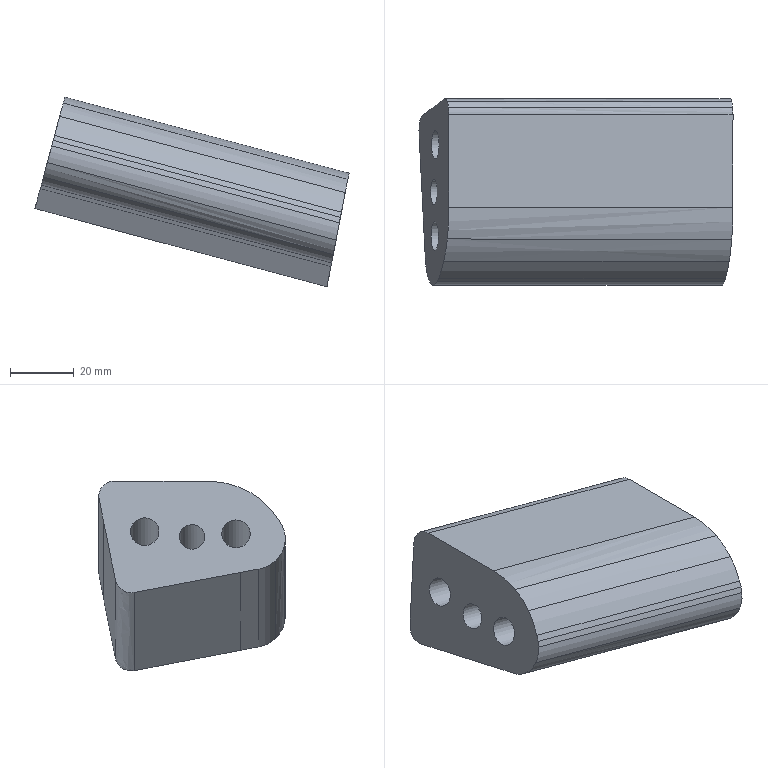Part | NX | features solid 2 | 1 solid | 30 faces | box 98.643 x 58.579 x 59.607 mm | volume 135226 mm3 | spline 16 | plane 8 | cylinder 6 | commonest cylinder face diameters 9.007 x2 14.508 x2 5.1 x1 8 x1
STEP:
#1=CARTESIAN_POINT('',(556.756,-84.584,-6.76));
#2=VERTEX_POINT('',#1);
#3=CARTESIAN_POINT('',(557.921,-84.584,-2.41));
#4=DIRECTION('',(-0.9659,-0.000000134,0.2588));
#5=DIRECTION('',(-0.2588,0.,-0.9659));
#6=AXIS2_PLACEMENT_3D('',#3,#4,#5);
#7=CIRCLE('',#6,4.503);
#8=EDGE_CURVE('',#2,#2,#7,.F.);
#9=ORIENTED_EDGE('',*,*,#8,.F.);
#10=EDGE_LOOP('',(#9));
#11=FACE_BOUND('',#10,.T.);
#12=CARTESIAN_POINT('',(558.279,-91.705,-1.074));
#13=VERTEX_POINT('',#12);
#14=CARTESIAN_POINT('',(557.921,-84.584,-2.41));
#15=DIRECTION('',(-0.9659,-0.000000134,0.2588));
#16=DIRECTION('',(0.04935,-0.9817,0.1842));
#17=AXIS2_PLACEMENT_3D('',#14,#15,#16);
#18=CIRCLE('',#17,7.254);
#19=EDGE_CURVE('',#13,#13,#18,.F.);
#20=ORIENTED_EDGE('',*,*,#19,.T.);
#21=EDGE_LOOP('',(#20));
#22=FACE_BOUND('',#21,.T.);
#23=CARTESIAN_POINT('',(557.921,-84.584,-2.41));
#24=DIRECTION('',(0.9659,0.000000134,-0.2588));
#25=DIRECTION('',(-0.2588,0.,-0.9659));
#26=AXIS2_PLACEMENT_3D('',#23,#24,#25);
#27=PLANE('',#26);
#28=ADVANCED_FACE('',(#11,#22),#27,.T.);
#29=CARTESIAN_POINT('',(583.419,-84.556,-16.752));
#30=VERTEX_POINT('',#29);
#31=CARTESIAN_POINT('',(584.806,-84.584,-9.614));
#32=DIRECTION('',(-0.9816,0.0002628,0.1908));
#33=DIRECTION('',(-0.1908,0.003761,-0.9816));
#34=AXIS2_PLACEMENT_3D('',#31,#32,#33);
#35=ELLIPSE('',#34,7.272,7.254);
#36=EDGE_CURVE('',#30,#30,#35,.F.);
#37=ORIENTED_EDGE('',*,*,#36,.T.);
#38=EDGE_LOOP('',(#37));
#39=FACE_BOUND('',#38,.T.);
#40=ORIENTED_EDGE('',*,*,#19,.F.);
#41=EDGE_LOOP('',(#40));
#42=FACE_BOUND('',#41,.T.);
#43=CARTESIAN_POINT('',(557.921,-84.584,-2.41));
#44=DIRECTION('',(0.9659,0.000000134,-0.2588));
#45=DIRECTION('',(-0.2588,0.,-0.9659));
#46=AXIS2_PLACEMENT_3D('',#43,#44,#45);
#47=CYLINDRICAL_SURFACE('',#46,7.254);
#48=ADVANCED_FACE('',(#39,#42),#47,.F.);
#49=ORIENTED_EDGE('',*,*,#36,.F.);
#50=EDGE_LOOP('',(#49));
#51=FACE_BOUND('',#50,.T.);
#52=CARTESIAN_POINT('',(583.557,-55.874,-16.077));
#53=VERTEX_POINT('',#52);
#54=CARTESIAN_POINT('',(584.945,-55.901,-8.939));
#55=DIRECTION('',(-0.9816,0.0002628,0.1908));
#56=DIRECTION('',(-0.1908,0.003761,-0.9816));
#57=AXIS2_PLACEMENT_3D('',#54,#55,#56);
#58=ELLIPSE('',#57,7.272,7.254);
#59=EDGE_CURVE('',#53,#53,#58,.F.);
#60=ORIENTED_EDGE('',*,*,#59,.F.);
#61=EDGE_LOOP('',(#60));
#62=FACE_BOUND('',#61,.T.);
#63=CARTESIAN_POINT('',(587.981,-44.117,6.663));
#64=VERTEX_POINT('',#63);
#65=CARTESIAN_POINT('',(588.09,-46.498,7.229));
#66=VERTEX_POINT('',#65);
#67=CARTESIAN_POINT('',(587.981,-44.117,6.663));
#68=CARTESIAN_POINT('',(588.053,-44.854,7.038));
#69=CARTESIAN_POINT('',(588.091,-45.668,7.229));
#70=CARTESIAN_POINT('',(588.09,-46.498,7.229));
#71=B_SPLINE_CURVE_WITH_KNOTS('',3,(#67,#68,#69,#70),.UNSPECIFIED.,.F.,.F.,(4,4),(0.,0.002457),.UNSPECIFIED.);
#72=EDGE_CURVE('',#64,#66,#71,.T.);
#73=ORIENTED_EDGE('',*,*,#72,.T.);
#74=CARTESIAN_POINT('',(588.08,-75.541,7.214));
#75=VERTEX_POINT('',#74);
#76=CARTESIAN_POINT('',(588.08,-75.571,7.214));
#77=DIRECTION('',(0.0003677,1.,0.000514));
#78=VECTOR('',#77,1000.);
#79=LINE('',#76,#78);
#80=EDGE_CURVE('',#75,#66,#79,.T.);
#81=ORIENTED_EDGE('',*,*,#80,.F.);
#82=CARTESIAN_POINT('',(587.706,-85.562,5.309));
#83=VERTEX_POINT('',#82);
#84=CARTESIAN_POINT('',(588.08,-75.541,7.214));
#85=CARTESIAN_POINT('',(588.078,-79.006,7.212));
#86=CARTESIAN_POINT('',(587.955,-82.348,6.581));
#87=CARTESIAN_POINT('',(587.706,-85.562,5.309));
#88=B_SPLINE_CURVE_WITH_KNOTS('',3,(#84,#85,#86,#87),.UNSPECIFIED.,.F.,.F.,(4,4),(0.,0.01021),.UNSPECIFIED.);
#89=EDGE_CURVE('',#75,#83,#88,.T.);
#90=ORIENTED_EDGE('',*,*,#89,.T.);
#91=CARTESIAN_POINT('',(586.892,-92.585,1.127));
#92=VERTEX_POINT('',#91);
#93=CARTESIAN_POINT('',(587.706,-85.562,5.309));
#94=CARTESIAN_POINT('',(587.508,-88.136,4.29));
#95=CARTESIAN_POINT('',(587.237,-90.477,2.898));
#96=CARTESIAN_POINT('',(586.892,-92.585,1.127));
#97=B_SPLINE_CURVE_WITH_KNOTS('',3,(#93,#94,#95,#96),.UNSPECIFIED.,.F.,.F.,(4,4),(0.,0.008214),.UNSPECIFIED.);
#98=EDGE_CURVE('',#83,#92,#97,.T.);
#99=ORIENTED_EDGE('',*,*,#98,.T.);
#100=CARTESIAN_POINT('',(585.695,-97.948,-5.022));
#101=VERTEX_POINT('',#100);
#102=CARTESIAN_POINT('',(586.892,-92.585,1.127));
#103=CARTESIAN_POINT('',(586.546,-94.699,-0.6484));
#104=CARTESIAN_POINT('',(586.147,-96.484,-2.701));
#105=CARTESIAN_POINT('',(585.695,-97.948,-5.022));
#106=B_SPLINE_CURVE_WITH_KNOTS('',3,(#102,#103,#104,#105),.UNSPECIFIED.,.F.,.F.,(4,4),(0.,0.008246),.UNSPECIFIED.);
#107=EDGE_CURVE('',#92,#101,#106,.T.);
#108=ORIENTED_EDGE('',*,*,#107,.T.);
#109=CARTESIAN_POINT('',(585.383,-98.902,-6.628));
#110=VERTEX_POINT('',#109);
#111=CARTESIAN_POINT('',(585.695,-97.948,-5.022));
#112=CARTESIAN_POINT('',(585.593,-98.28,-5.549));
#113=CARTESIAN_POINT('',(585.488,-98.598,-6.085));
#114=CARTESIAN_POINT('',(585.383,-98.902,-6.628));
#115=B_SPLINE_CURVE_WITH_KNOTS('',3,(#111,#112,#113,#114),.UNSPECIFIED.,.F.,.F.,(4,4),(0.,0.001895),.UNSPECIFIED.);
#116=EDGE_CURVE('',#101,#110,#115,.T.);
#117=ORIENTED_EDGE('',*,*,#116,.T.);
#118=CARTESIAN_POINT('',(585.05,-99.633,-8.337));
#119=VERTEX_POINT('',#118);
#120=CARTESIAN_POINT('',(585.383,-98.902,-6.628));
#121=CARTESIAN_POINT('',(585.277,-99.207,-7.173));
#122=CARTESIAN_POINT('',(585.166,-99.451,-7.742));
#123=CARTESIAN_POINT('',(585.05,-99.633,-8.337));
#124=B_SPLINE_CURVE_WITH_KNOTS('',3,(#120,#121,#122,#123),.UNSPECIFIED.,.F.,.F.,(4,4),(0.,0.001887),.UNSPECIFIED.);
#125=EDGE_CURVE('',#110,#119,#124,.T.);
#126=ORIENTED_EDGE('',*,*,#125,.T.);
#127=CARTESIAN_POINT('',(584.005,-99.734,-13.713));
#128=VERTEX_POINT('',#127);
#129=CARTESIAN_POINT('',(584.005,-99.734,-13.713));
#130=CARTESIAN_POINT('',(584.349,-100.208,-11.945));
#131=CARTESIAN_POINT('',(584.71,-100.172,-10.087));
#132=CARTESIAN_POINT('',(585.05,-99.633,-8.337));
#133=B_SPLINE_CURVE_WITH_KNOTS('',3,(#129,#130,#131,#132),.UNSPECIFIED.,.F.,.F.,(4,4),(0.,0.00551),.UNSPECIFIED.);
#134=EDGE_CURVE('',#128,#119,#133,.T.);
#135=ORIENTED_EDGE('',*,*,#134,.F.);
#136=CARTESIAN_POINT('',(583.108,-96.945,-18.332));
#137=VERTEX_POINT('',#136);
#138=CARTESIAN_POINT('',(584.005,-99.734,-13.713));
#139=CARTESIAN_POINT('',(583.662,-99.26,-15.479));
#140=CARTESIAN_POINT('',(583.352,-98.295,-17.076));
#141=CARTESIAN_POINT('',(583.108,-96.945,-18.332));
#142=B_SPLINE_CURVE_WITH_KNOTS('',3,(#138,#139,#140,#141),.UNSPECIFIED.,.F.,.F.,(4,4),(0.,0.005502),.UNSPECIFIED.);
#143=EDGE_CURVE('',#128,#137,#142,.T.);
#144=ORIENTED_EDGE('',*,*,#143,.T.);
#145=CARTESIAN_POINT('',(582.61,-91.803,-20.901));
#146=VERTEX_POINT('',#145);
#147=CARTESIAN_POINT('',(583.108,-96.945,-18.332));
#148=CARTESIAN_POINT('',(582.851,-95.518,-19.658));
#149=CARTESIAN_POINT('',(582.678,-93.734,-20.549));
#150=CARTESIAN_POINT('',(582.61,-91.803,-20.901));
#151=B_SPLINE_CURVE_WITH_KNOTS('',3,(#147,#148,#149,#150),.UNSPECIFIED.,.F.,.F.,(4,4),(0.,0.005811),.UNSPECIFIED.);
#152=EDGE_CURVE('',#137,#146,#151,.T.);
#153=ORIENTED_EDGE('',*,*,#152,.T.);
#154=CARTESIAN_POINT('',(582.397,-85.892,-22.005));
#155=VERTEX_POINT('',#154);
#156=CARTESIAN_POINT('',(582.61,-91.803,-20.901));
#157=CARTESIAN_POINT('',(582.541,-89.831,-21.261));
#158=CARTESIAN_POINT('',(582.47,-87.86,-21.628));
#159=CARTESIAN_POINT('',(582.397,-85.892,-22.005));
#160=B_SPLINE_CURVE_WITH_KNOTS('',3,(#156,#157,#158,#159),.UNSPECIFIED.,.F.,.F.,(4,4),(0.,0.006017),.UNSPECIFIED.);
#161=EDGE_CURVE('',#146,#155,#160,.T.);
#162=ORIENTED_EDGE('',*,*,#161,.T.);
#163=CARTESIAN_POINT('',(581.168,-52.586,-28.373));
#164=VERTEX_POINT('',#163);
#165=CARTESIAN_POINT('',(573.42,157.396,-68.523));
#166=DIRECTION('',(-0.03622,0.9816,-0.1877));
#167=VECTOR('',#166,1000.);
#168=LINE('',#165,#167);
#169=EDGE_CURVE('',#155,#164,#168,.T.);
#170=ORIENTED_EDGE('',*,*,#169,.T.);
#171=CARTESIAN_POINT('',(581.924,-46.723,-24.494));
#172=VERTEX_POINT('',#171);
#173=CARTESIAN_POINT('',(581.168,-52.586,-28.373));
#174=CARTESIAN_POINT('',(581.12,-51.29,-28.621));
#175=CARTESIAN_POINT('',(581.23,-48.542,-28.06));
#176=CARTESIAN_POINT('',(581.677,-46.975,-25.766));
#177=CARTESIAN_POINT('',(581.924,-46.723,-24.494));
#178=B_SPLINE_CURVE_WITH_KNOTS('',3,(#173,#174,#175,#176,#177),.UNSPECIFIED.,.F.,.F.,(4,1,4),(0.,0.003905,0.007811),.UNSPECIFIED.);
#179=EDGE_CURVE('',#164,#172,#178,.T.);
#180=ORIENTED_EDGE('',*,*,#179,.T.);
#181=CARTESIAN_POINT('',(584.195,-44.406,-12.814));
#182=VERTEX_POINT('',#181);
#183=CARTESIAN_POINT('',(585.983,-42.581,-3.616));
#184=DIRECTION('',(-0.1873,-0.1911,-0.9635));
#185=VECTOR('',#184,1000.);
#186=LINE('',#183,#185);
#187=EDGE_CURVE('',#182,#172,#186,.T.);
#188=ORIENTED_EDGE('',*,*,#187,.F.);
#189=CARTESIAN_POINT('',(585.604,-42.975,-5.566));
#190=VERTEX_POINT('',#189);
#191=CARTESIAN_POINT('',(584.195,-44.406,-12.814));
#192=CARTESIAN_POINT('',(584.665,-43.926,-10.398));
#193=CARTESIAN_POINT('',(585.134,-43.45,-7.982));
#194=CARTESIAN_POINT('',(585.604,-42.975,-5.566));
#195=B_SPLINE_CURVE_WITH_KNOTS('',3,(#191,#192,#193,#194),.UNSPECIFIED.,.F.,.F.,(4,4),(0.,0.007522),.UNSPECIFIED.);
#196=EDGE_CURVE('',#182,#190,#195,.T.);
#197=ORIENTED_EDGE('',*,*,#196,.T.);
#198=CARTESIAN_POINT('',(587.,-41.572,1.616));
#199=VERTEX_POINT('',#198);
#200=CARTESIAN_POINT('',(585.604,-42.975,-5.566));
#201=CARTESIAN_POINT('',(586.07,-42.505,-3.172));
#202=CARTESIAN_POINT('',(586.535,-42.037,-0.7783));
#203=CARTESIAN_POINT('',(587.,-41.572,1.616));
#204=B_SPLINE_CURVE_WITH_KNOTS('',3,(#200,#201,#202,#203),.UNSPECIFIED.,.F.,.F.,(4,4),(0.,0.007449),.UNSPECIFIED.);
#205=EDGE_CURVE('',#190,#199,#204,.T.);
#206=ORIENTED_EDGE('',*,*,#205,.T.);
#207=CARTESIAN_POINT('',(587.353,-41.584,3.431));
#208=VERTEX_POINT('',#207);
#209=CARTESIAN_POINT('',(587.,-41.572,1.616));
#210=CARTESIAN_POINT('',(587.118,-41.454,2.222));
#211=CARTESIAN_POINT('',(587.236,-41.457,2.827));
#212=CARTESIAN_POINT('',(587.353,-41.584,3.431));
#213=B_SPLINE_CURVE_WITH_KNOTS('',3,(#209,#210,#211,#212),.UNSPECIFIED.,.F.,.F.,(4,4),(0.,0.001849),.UNSPECIFIED.);
#214=EDGE_CURVE('',#199,#208,#213,.T.);
#215=ORIENTED_EDGE('',*,*,#214,.T.);
#216=CARTESIAN_POINT('',(587.677,-42.305,5.095));
#217=VERTEX_POINT('',#216);
#218=CARTESIAN_POINT('',(587.353,-41.584,3.431));
#219=CARTESIAN_POINT('',(587.47,-41.711,4.033));
#220=CARTESIAN_POINT('',(587.578,-41.952,4.588));
#221=CARTESIAN_POINT('',(587.677,-42.305,5.095));
#222=B_SPLINE_CURVE_WITH_KNOTS('',3,(#218,#219,#220,#221),.UNSPECIFIED.,.F.,.F.,(4,4),(0.,0.001842),.UNSPECIFIED.);
#223=EDGE_CURVE('',#208,#217,#222,.T.);
#224=ORIENTED_EDGE('',*,*,#223,.T.);
#225=CARTESIAN_POINT('',(587.677,-42.305,5.095));
#226=CARTESIAN_POINT('',(587.806,-42.767,5.759));
#227=CARTESIAN_POINT('',(587.909,-43.389,6.293));
#228=CARTESIAN_POINT('',(587.981,-44.117,6.663));
#229=B_SPLINE_CURVE_WITH_KNOTS('',3,(#225,#226,#227,#228),.UNSPECIFIED.,.F.,.F.,(4,4),(0.,0.002422),.UNSPECIFIED.);
#230=EDGE_CURVE('',#217,#64,#229,.T.);
#231=ORIENTED_EDGE('',*,*,#230,.T.);
#232=EDGE_LOOP('',(#73,#81,#90,#99,#108,#117,#126,#135,#144,#153,#162,#170,#180,#188,#197,#206,#215,#224,#231));
#233=FACE_BOUND('',#232,.T.);
#234=CARTESIAN_POINT('',(585.102,-70.813,-8.111));
#235=VERTEX_POINT('',#234);
#236=CARTESIAN_POINT('',(584.614,-70.804,-10.62));
#237=DIRECTION('',(-0.9816,0.0002628,0.1908));
#238=DIRECTION('',(0.1908,-0.003761,0.9816));
#239=AXIS2_PLACEMENT_3D('',#236,#237,#238);
#240=ELLIPSE('',#239,2.556,2.55);
#241=EDGE_CURVE('',#235,#235,#240,.F.);
#242=ORIENTED_EDGE('',*,*,#241,.F.);
#243=EDGE_LOOP('',(#242));
#244=FACE_BOUND('',#243,.T.);
#245=CARTESIAN_POINT('',(574.049,158.037,-65.289));
#246=DIRECTION('',(-0.9816,0.0002628,0.1908));
#247=DIRECTION('',(0.1908,0.001526,0.9816));
#248=AXIS2_PLACEMENT_3D('',#245,#246,#247);
#249=PLANE('',#248);
#250=ADVANCED_FACE('',(#51,#62,#233,#244),#249,.F.);
#251=CARTESIAN_POINT('',(493.104,-70.804,9.759));
#252=VERTEX_POINT('',#251);
#253=CARTESIAN_POINT('',(494.139,-70.804,13.623));
#254=DIRECTION('',(-0.9659,-0.000000134,0.2588));
#255=DIRECTION('',(-0.2588,0.,-0.9659));
#256=AXIS2_PLACEMENT_3D('',#253,#254,#255);
#257=CIRCLE('',#256,4.);
#258=EDGE_CURVE('',#252,#252,#257,.T.);
#259=ORIENTED_EDGE('',*,*,#258,.F.);
#260=EDGE_LOOP('',(#259));
#261=FACE_BOUND('',#260,.T.);
#262=CARTESIAN_POINT('',(495.747,-55.901,19.624));
#263=VERTEX_POINT('',#262);
#264=CARTESIAN_POINT('',(494.581,-55.901,15.274));
#265=DIRECTION('',(0.9659,0.000000134,-0.2588));
#266=DIRECTION('',(0.2588,0.,0.9659));
#267=AXIS2_PLACEMENT_3D('',#264,#265,#266);
#268=CIRCLE('',#267,4.503);
#269=EDGE_CURVE('',#263,#263,#268,.T.);
#270=ORIENTED_EDGE('',*,*,#269,.T.);
#271=EDGE_LOOP('',(#270));
#272=FACE_BOUND('',#271,.T.);
#273=CARTESIAN_POINT('',(493.562,-44.406,11.471));
#274=VERTEX_POINT('',#273);
#275=CARTESIAN_POINT('',(495.469,-42.975,18.586));
#276=VERTEX_POINT('',#275);
#277=CARTESIAN_POINT('',(493.562,-44.406,11.471));
#278=CARTESIAN_POINT('',(494.198,-43.926,13.842));
#279=CARTESIAN_POINT('',(494.833,-43.45,16.214));
#280=CARTESIAN_POINT('',(495.469,-42.975,18.586));
#281=B_SPLINE_CURVE_WITH_KNOTS('',3,(#277,#278,#279,#280),.UNSPECIFIED.,.F.,.F.,(4,4),(0.,0.007504),.UNSPECIFIED.);
#282=EDGE_CURVE('',#274,#276,#281,.T.);
#283=ORIENTED_EDGE('',*,*,#282,.F.);
#284=CARTESIAN_POINT('',(490.49,-46.723,0.005664));
#285=VERTEX_POINT('',#284);
#286=CARTESIAN_POINT('',(493.562,-44.406,11.471));
#287=DIRECTION('',(-0.254,-0.1916,-0.948));
#288=VECTOR('',#287,1000.);
#289=LINE('',#286,#288);
#290=EDGE_CURVE('',#274,#285,#289,.T.);
#291=ORIENTED_EDGE('',*,*,#290,.T.);
#292=CARTESIAN_POINT('',(489.47,-52.586,-3.803));
#293=VERTEX_POINT('',#292);
#294=CARTESIAN_POINT('',(490.49,-46.723,0.005664));
#295=CARTESIAN_POINT('',(490.155,-46.976,-1.245));
#296=CARTESIAN_POINT('',(489.553,-48.54,-3.493));
#297=CARTESIAN_POINT('',(489.405,-51.291,-4.046));
#298=CARTESIAN_POINT('',(489.47,-52.586,-3.803));
#299=B_SPLINE_CURVE_WITH_KNOTS('',3,(#294,#295,#296,#297,#298),.UNSPECIFIED.,.F.,.F.,(4,1,4),(0.,0.003902,0.007804),.UNSPECIFIED.);
#300=EDGE_CURVE('',#285,#293,#299,.T.);
#301=ORIENTED_EDGE('',*,*,#300,.T.);
#302=CARTESIAN_POINT('',(491.144,-85.892,2.446));
#303=VERTEX_POINT('',#302);
#304=CARTESIAN_POINT('',(489.47,-52.586,-3.803));
#305=DIRECTION('',(0.04935,-0.9817,0.1842));
#306=VECTOR('',#305,1000.);
#307=LINE('',#304,#306);
#308=EDGE_CURVE('',#293,#303,#307,.T.);
#309=ORIENTED_EDGE('',*,*,#308,.T.);
#310=CARTESIAN_POINT('',(491.435,-91.803,3.529));
#311=VERTEX_POINT('',#310);
#312=CARTESIAN_POINT('',(491.144,-85.892,2.446));
#313=CARTESIAN_POINT('',(491.243,-87.86,2.816));
#314=CARTESIAN_POINT('',(491.34,-89.831,3.177));
#315=CARTESIAN_POINT('',(491.435,-91.803,3.529));
#316=B_SPLINE_CURVE_WITH_KNOTS('',3,(#312,#313,#314,#315),.UNSPECIFIED.,.F.,.F.,(4,4),(0.,0.006016),.UNSPECIFIED.);
#317=EDGE_CURVE('',#303,#311,#316,.T.);
#318=ORIENTED_EDGE('',*,*,#317,.T.);
#319=CARTESIAN_POINT('',(492.11,-96.945,6.051));
#320=VERTEX_POINT('',#319);
#321=CARTESIAN_POINT('',(492.11,-96.945,6.051));
#322=CARTESIAN_POINT('',(491.761,-95.517,4.748));
#323=CARTESIAN_POINT('',(491.527,-93.734,3.874));
#324=CARTESIAN_POINT('',(491.435,-91.803,3.529));
#325=B_SPLINE_CURVE_WITH_KNOTS('',3,(#321,#322,#323,#324),.UNSPECIFIED.,.F.,.F.,(4,4),(0.,0.005808),.UNSPECIFIED.);
#326=EDGE_CURVE('',#320,#311,#325,.T.);
#327=ORIENTED_EDGE('',*,*,#326,.F.);
#328=CARTESIAN_POINT('',(493.325,-99.734,10.584));
#329=VERTEX_POINT('',#328);
#330=CARTESIAN_POINT('',(492.11,-96.945,6.051));
#331=CARTESIAN_POINT('',(492.44,-98.295,7.283));
#332=CARTESIAN_POINT('',(492.86,-99.26,8.85));
#333=CARTESIAN_POINT('',(493.325,-99.734,10.584));
#334=B_SPLINE_CURVE_WITH_KNOTS('',3,(#330,#331,#332,#333),.UNSPECIFIED.,.F.,.F.,(4,4),(0.,0.005492),.UNSPECIFIED.);
#335=EDGE_CURVE('',#320,#329,#334,.T.);
#336=ORIENTED_EDGE('',*,*,#335,.T.);
#337=CARTESIAN_POINT('',(494.739,-99.633,15.862));
#338=VERTEX_POINT('',#337);
#339=CARTESIAN_POINT('',(493.325,-99.734,10.584));
#340=CARTESIAN_POINT('',(493.79,-100.208,12.32));
#341=CARTESIAN_POINT('',(494.279,-100.172,14.144));
#342=CARTESIAN_POINT('',(494.739,-99.633,15.862));
#343=B_SPLINE_CURVE_WITH_KNOTS('',3,(#339,#340,#341,#342),.UNSPECIFIED.,.F.,.F.,(4,4),(0.,0.005497),.UNSPECIFIED.);
#344=EDGE_CURVE('',#329,#338,#343,.T.);
#345=ORIENTED_EDGE('',*,*,#344,.T.);
#346=CARTESIAN_POINT('',(495.188,-98.902,17.539));
#347=VERTEX_POINT('',#346);
#348=CARTESIAN_POINT('',(494.739,-99.633,15.862));
#349=CARTESIAN_POINT('',(494.896,-99.451,16.446));
#350=CARTESIAN_POINT('',(495.045,-99.207,17.005));
#351=CARTESIAN_POINT('',(495.188,-98.902,17.539));
#352=B_SPLINE_CURVE_WITH_KNOTS('',3,(#348,#349,#350,#351),.UNSPECIFIED.,.F.,.F.,(4,4),(0.,0.001884),.UNSPECIFIED.);
#353=EDGE_CURVE('',#338,#347,#352,.T.);
#354=ORIENTED_EDGE('',*,*,#353,.T.);
#355=CARTESIAN_POINT('',(495.611,-97.948,19.116));
#356=VERTEX_POINT('',#355);
#357=CARTESIAN_POINT('',(495.188,-98.902,17.539));
#358=CARTESIAN_POINT('',(495.331,-98.598,18.073));
#359=CARTESIAN_POINT('',(495.472,-98.28,18.598));
#360=CARTESIAN_POINT('',(495.611,-97.948,19.116));
#361=B_SPLINE_CURVE_WITH_KNOTS('',3,(#357,#358,#359,#360),.UNSPECIFIED.,.F.,.F.,(4,4),(0.,0.001891),.UNSPECIFIED.);
#362=EDGE_CURVE('',#347,#356,#361,.T.);
#363=ORIENTED_EDGE('',*,*,#362,.T.);
#364=CARTESIAN_POINT('',(497.228,-92.585,25.152));
#365=VERTEX_POINT('',#364);
#366=CARTESIAN_POINT('',(495.611,-97.948,19.116));
#367=CARTESIAN_POINT('',(496.222,-96.483,21.396));
#368=CARTESIAN_POINT('',(496.762,-94.698,23.41));
#369=CARTESIAN_POINT('',(497.228,-92.585,25.152));
#370=B_SPLINE_CURVE_WITH_KNOTS('',3,(#366,#367,#368,#369),.UNSPECIFIED.,.F.,.F.,(4,4),(0.,0.008235),.UNSPECIFIED.);
#371=EDGE_CURVE('',#356,#365,#370,.T.);
#372=ORIENTED_EDGE('',*,*,#371,.T.);
#373=CARTESIAN_POINT('',(498.328,-85.563,29.257));
#374=VERTEX_POINT('',#373);
#375=CARTESIAN_POINT('',(497.228,-92.585,25.152));
#376=CARTESIAN_POINT('',(497.694,-90.477,26.891));
#377=CARTESIAN_POINT('',(498.061,-88.135,28.258));
#378=CARTESIAN_POINT('',(498.328,-85.563,29.257));
#379=B_SPLINE_CURVE_WITH_KNOTS('',3,(#375,#376,#377,#378),.UNSPECIFIED.,.F.,.F.,(4,4),(0.,0.008209),.UNSPECIFIED.);
#380=EDGE_CURVE('',#365,#374,#379,.T.);
#381=ORIENTED_EDGE('',*,*,#380,.T.);
#382=CARTESIAN_POINT('',(498.83,-75.541,31.128));
#383=VERTEX_POINT('',#382);
#384=CARTESIAN_POINT('',(498.83,-75.541,31.128));
#385=CARTESIAN_POINT('',(498.829,-79.006,31.127));
#386=CARTESIAN_POINT('',(498.663,-82.347,30.507));
#387=CARTESIAN_POINT('',(498.328,-85.563,29.257));
#388=B_SPLINE_CURVE_WITH_KNOTS('',3,(#384,#385,#386,#387),.UNSPECIFIED.,.F.,.F.,(4,4),(0.,0.01021),.UNSPECIFIED.);
#389=EDGE_CURVE('',#383,#374,#388,.T.);
#390=ORIENTED_EDGE('',*,*,#389,.F.);
#391=CARTESIAN_POINT('',(498.834,-46.498,31.145));
#392=VERTEX_POINT('',#391);
#393=CARTESIAN_POINT('',(498.83,-75.541,31.128));
#394=DIRECTION('',(0.000153,1.,0.0005715));
#395=VECTOR('',#394,1000.);
#396=LINE('',#393,#395);
#397=EDGE_CURVE('',#383,#392,#396,.T.);
#398=ORIENTED_EDGE('',*,*,#397,.T.);
#399=CARTESIAN_POINT('',(498.685,-44.117,30.589));
#400=VERTEX_POINT('',#399);
#401=CARTESIAN_POINT('',(498.834,-46.498,31.145));
#402=CARTESIAN_POINT('',(498.834,-45.668,31.146));
#403=CARTESIAN_POINT('',(498.784,-44.855,30.957));
#404=CARTESIAN_POINT('',(498.685,-44.117,30.589));
#405=B_SPLINE_CURVE_WITH_KNOTS('',3,(#401,#402,#403,#404),.UNSPECIFIED.,.F.,.F.,(4,4),(0.,0.002456),.UNSPECIFIED.);
#406=EDGE_CURVE('',#392,#400,#405,.T.);
#407=ORIENTED_EDGE('',*,*,#406,.T.);
#408=CARTESIAN_POINT('',(498.273,-42.305,29.051));
#409=VERTEX_POINT('',#408);
#410=CARTESIAN_POINT('',(498.685,-44.117,30.589));
#411=CARTESIAN_POINT('',(498.588,-43.39,30.227));
#412=CARTESIAN_POINT('',(498.448,-42.767,29.703));
#413=CARTESIAN_POINT('',(498.273,-42.305,29.051));
#414=B_SPLINE_CURVE_WITH_KNOTS('',3,(#410,#411,#412,#413),.UNSPECIFIED.,.F.,.F.,(4,4),(0.,0.00242),.UNSPECIFIED.);
#415=EDGE_CURVE('',#400,#409,#414,.T.);
#416=ORIENTED_EDGE('',*,*,#415,.T.);
#417=CARTESIAN_POINT('',(497.835,-41.584,27.417));
#418=VERTEX_POINT('',#417);
#419=CARTESIAN_POINT('',(498.273,-42.305,29.051));
#420=CARTESIAN_POINT('',(498.14,-41.952,28.553));
#421=CARTESIAN_POINT('',(497.994,-41.711,28.008));
#422=CARTESIAN_POINT('',(497.835,-41.584,27.417));
#423=B_SPLINE_CURVE_WITH_KNOTS('',3,(#419,#420,#421,#422),.UNSPECIFIED.,.F.,.F.,(4,4),(0.,0.001839),.UNSPECIFIED.);
#424=EDGE_CURVE('',#409,#418,#423,.T.);
#425=ORIENTED_EDGE('',*,*,#424,.T.);
#426=CARTESIAN_POINT('',(497.358,-41.572,25.636));
#427=VERTEX_POINT('',#426);
#428=CARTESIAN_POINT('',(497.835,-41.584,27.417));
#429=CARTESIAN_POINT('',(497.676,-41.457,26.824));
#430=CARTESIAN_POINT('',(497.517,-41.454,26.23));
#431=CARTESIAN_POINT('',(497.358,-41.572,25.636));
#432=B_SPLINE_CURVE_WITH_KNOTS('',3,(#428,#429,#430,#431),.UNSPECIFIED.,.F.,.F.,(4,4),(0.,0.001844),.UNSPECIFIED.);
#433=EDGE_CURVE('',#418,#427,#432,.T.);
#434=ORIENTED_EDGE('',*,*,#433,.T.);
#435=CARTESIAN_POINT('',(497.358,-41.572,25.636));
#436=CARTESIAN_POINT('',(496.728,-42.037,23.285));
#437=CARTESIAN_POINT('',(496.099,-42.505,20.935));
#438=CARTESIAN_POINT('',(495.469,-42.975,18.586));
#439=B_SPLINE_CURVE_WITH_KNOTS('',3,(#435,#436,#437,#438),.UNSPECIFIED.,.F.,.F.,(4,4),(0.,0.007432),.UNSPECIFIED.);
#440=EDGE_CURVE('',#427,#276,#439,.T.);
#441=ORIENTED_EDGE('',*,*,#440,.T.);
#442=EDGE_LOOP('',(#283,#291,#301,#309,#318,#327,#336,#345,#354,#363,#372,#381,#390,#398,#407,#416,#425,#434,#441));
#443=FACE_BOUND('',#442,.T.);
#444=CARTESIAN_POINT('',(495.569,-84.584,18.96));
#445=VERTEX_POINT('',#444);
#446=CARTESIAN_POINT('',(494.404,-84.584,14.61));
#447=DIRECTION('',(0.9659,0.000000134,-0.2588));
#448=DIRECTION('',(0.2588,0.,0.9659));
#449=AXIS2_PLACEMENT_3D('',#446,#447,#448);
#450=CIRCLE('',#449,4.503);
#451=EDGE_CURVE('',#445,#445,#450,.T.);
#452=ORIENTED_EDGE('',*,*,#451,.T.);
#453=EDGE_LOOP('',(#452));
#454=FACE_BOUND('',#453,.T.);
#455=CARTESIAN_POINT('',(327.709,4.191,-607.503));
#456=DIRECTION('',(-0.9659,-0.000000134,0.2588));
#457=DIRECTION('',(0.2588,0.,0.9659));
#458=AXIS2_PLACEMENT_3D('',#455,#456,#457);
#459=PLANE('',#458);
#460=ADVANCED_FACE('',(#261,#272,#443,#454),#459,.T.);
#461=ORIENTED_EDGE('',*,*,#451,.F.);
#462=EDGE_LOOP('',(#461));
#463=FACE_BOUND('',#462,.T.);
#464=ORIENTED_EDGE('',*,*,#8,.T.);
#465=EDGE_LOOP('',(#464));
#466=FACE_BOUND('',#465,.T.);
#467=CARTESIAN_POINT('',(607.183,-84.584,-15.61));
#468=DIRECTION('',(-0.9659,-0.000000134,0.2588));
#469=DIRECTION('',(0.2588,0.,0.9659));
#470=AXIS2_PLACEMENT_3D('',#467,#468,#469);
#471=CYLINDRICAL_SURFACE('',#470,4.503);
#472=ADVANCED_FACE('',(#463,#466),#471,.F.);
#473=CARTESIAN_POINT('',(457.154,-46.498,42.313));
#474=DIRECTION('',(0.9659,0.000000134,-0.2588));
#475=VECTOR('',#474,1000.);
#476=LINE('',#473,#475);
#477=EDGE_CURVE('',#66,#392,#476,.F.);
#478=ORIENTED_EDGE('',*,*,#477,.T.);
#479=ORIENTED_EDGE('',*,*,#397,.F.);
#480=CARTESIAN_POINT('',(457.088,-75.541,42.313));
#481=DIRECTION('',(0.9659,0.000000134,-0.2588));
#482=VECTOR('',#481,1000.);
#483=LINE('',#480,#482);
#484=EDGE_CURVE('',#75,#383,#483,.F.);
#485=ORIENTED_EDGE('',*,*,#484,.F.);
#486=ORIENTED_EDGE('',*,*,#80,.T.);
#487=EDGE_LOOP('',(#478,#479,#485,#486));
#488=FACE_BOUND('',#487,.T.);
#489=CARTESIAN_POINT('',(457.088,-75.541,42.313));
#490=DIRECTION('',(0.2588,-0.0005916,0.9659));
#491=DIRECTION('',(0.9659,0.,-0.2588));
#492=AXIS2_PLACEMENT_3D('',#489,#490,#491);
#493=PLANE('',#492);
#494=ADVANCED_FACE('',(#488),#493,.T.);
#495=CARTESIAN_POINT('',(455.12,-41.584,38.862));
#496=DIRECTION('',(0.9659,0.000000134,-0.2588));
#497=VECTOR('',#496,1000.);
#498=LINE('',#495,#497);
#499=EDGE_CURVE('',#208,#418,#498,.F.);
#500=ORIENTED_EDGE('',*,*,#499,.T.);
#501=ORIENTED_EDGE('',*,*,#424,.F.);
#502=CARTESIAN_POINT('',(455.997,-42.305,40.379));
#503=DIRECTION('',(0.9659,0.000000134,-0.2588));
#504=VECTOR('',#503,1000.);
#505=LINE('',#502,#504);
#506=EDGE_CURVE('',#217,#409,#505,.F.);
#507=ORIENTED_EDGE('',*,*,#506,.F.);
#508=ORIENTED_EDGE('',*,*,#223,.F.);
#509=EDGE_LOOP('',(#500,#501,#507,#508));
#510=FACE_BOUND('',#509,.T.);
#511=CARTESIAN_POINT('',(497.733,-42.305,29.195));
#512=CARTESIAN_POINT('',(588.77,-42.305,4.802));
#513=CARTESIAN_POINT('',(497.46,-41.956,28.741));
#514=CARTESIAN_POINT('',(588.497,-41.956,4.347));
#515=CARTESIAN_POINT('',(497.16,-41.709,28.223));
#516=CARTESIAN_POINT('',(588.197,-41.709,3.829));
#517=CARTESIAN_POINT('',(496.856,-41.584,27.679));
#518=CARTESIAN_POINT('',(587.893,-41.584,3.286));
#519=B_SPLINE_SURFACE_WITH_KNOTS('',3,1,((#511,#512),(#513,#514),(#515,#516),(#517,#518)),.SURF_OF_LINEAR_EXTRUSION.,.F.,.F.,.F.,(4,4),(2,2),(6.091,6.476),(0.,1.),.PIECEWISE_BEZIER_KNOTS.);
#520=ADVANCED_FACE('',(#510),#519,.F.);
#521=ORIENTED_EDGE('',*,*,#506,.T.);
#522=ORIENTED_EDGE('',*,*,#415,.F.);
#523=CARTESIAN_POINT('',(456.849,-44.117,41.799));
#524=DIRECTION('',(0.9659,0.000000134,-0.2588));
#525=VECTOR('',#524,1000.);
#526=LINE('',#523,#525);
#527=EDGE_CURVE('',#64,#400,#526,.F.);
#528=ORIENTED_EDGE('',*,*,#527,.F.);
#529=ORIENTED_EDGE('',*,*,#230,.F.);
#530=EDGE_LOOP('',(#521,#522,#528,#529));
#531=FACE_BOUND('',#530,.T.);
#532=CARTESIAN_POINT('',(498.146,-44.117,30.734));
#533=CARTESIAN_POINT('',(589.068,-44.117,6.371));
#534=CARTESIAN_POINT('',(497.945,-43.388,30.398));
#535=CARTESIAN_POINT('',(588.867,-43.388,6.035));
#536=CARTESIAN_POINT('',(497.65,-42.76,29.905));
#537=CARTESIAN_POINT('',(588.571,-42.76,5.542));
#538=CARTESIAN_POINT('',(497.294,-42.305,29.313));
#539=CARTESIAN_POINT('',(588.216,-42.305,4.951));
#540=B_SPLINE_SURFACE_WITH_KNOTS('',3,1,((#532,#533),(#534,#535),(#536,#537),(#538,#539)),.SURF_OF_LINEAR_EXTRUSION.,.F.,.F.,.F.,(4,4),(2,2),(0.7564,1.252),(0.,1.),.PIECEWISE_BEZIER_KNOTS.);
#541=ADVANCED_FACE('',(#531),#540,.F.);
#542=ORIENTED_EDGE('',*,*,#527,.T.);
#543=ORIENTED_EDGE('',*,*,#406,.F.);
#544=ORIENTED_EDGE('',*,*,#477,.F.);
#545=ORIENTED_EDGE('',*,*,#72,.F.);
#546=EDGE_LOOP('',(#542,#543,#544,#545));
#547=FACE_BOUND('',#546,.T.);
#548=CARTESIAN_POINT('',(498.296,-46.498,31.289));
#549=CARTESIAN_POINT('',(588.822,-46.498,7.033));
#550=CARTESIAN_POINT('',(498.298,-45.671,31.289));
#551=CARTESIAN_POINT('',(588.824,-45.671,7.033));
#552=CARTESIAN_POINT('',(498.192,-44.845,31.111));
#553=CARTESIAN_POINT('',(588.718,-44.845,6.855));
#554=CARTESIAN_POINT('',(497.992,-44.117,30.775));
#555=CARTESIAN_POINT('',(588.517,-44.117,6.519));
#556=B_SPLINE_SURFACE_WITH_KNOTS('',3,1,((#548,#549),(#550,#551),(#552,#553),(#554,#555)),.SURF_OF_LINEAR_EXTRUSION.,.F.,.F.,.F.,(4,4),(2,2),(0.2624,0.7564),(0.,1.),.PIECEWISE_BEZIER_KNOTS.);
#557=ADVANCED_FACE('',(#547),#556,.F.);
#558=ORIENTED_EDGE('',*,*,#484,.T.);
#559=ORIENTED_EDGE('',*,*,#389,.T.);
#560=CARTESIAN_POINT('',(456.027,-85.563,40.592));
#561=DIRECTION('',(0.9659,0.000000134,-0.2588));
#562=VECTOR('',#561,1000.);
#563=LINE('',#560,#562);
#564=EDGE_CURVE('',#83,#374,#563,.F.);
#565=ORIENTED_EDGE('',*,*,#564,.F.);
#566=ORIENTED_EDGE('',*,*,#89,.F.);
#567=EDGE_LOOP('',(#558,#559,#565,#566));
#568=FACE_BOUND('',#567,.T.);
#569=CARTESIAN_POINT('',(497.229,-85.563,29.552));
#570=CARTESIAN_POINT('',(588.246,-85.562,5.164));
#571=CARTESIAN_POINT('',(497.92,-82.399,30.684));
#572=CARTESIAN_POINT('',(588.936,-82.399,6.296));
#573=CARTESIAN_POINT('',(498.282,-78.971,31.273));
#574=CARTESIAN_POINT('',(589.299,-78.971,6.885));
#575=CARTESIAN_POINT('',(498.29,-75.541,31.273));
#576=CARTESIAN_POINT('',(589.307,-75.541,6.885));
#577=B_SPLINE_SURFACE_WITH_KNOTS('',3,1,((#569,#570),(#571,#572),(#573,#574),(#575,#576)),.SURF_OF_LINEAR_EXTRUSION.,.F.,.F.,.F.,(4,4),(2,2),(6.085,6.481),(0.,1.),.PIECEWISE_BEZIER_KNOTS.);
#578=ADVANCED_FACE('',(#568),#577,.F.);
#579=ORIENTED_EDGE('',*,*,#564,.T.);
#580=ORIENTED_EDGE('',*,*,#380,.F.);
#581=CARTESIAN_POINT('',(453.915,-92.585,36.758));
#582=DIRECTION('',(0.9659,0.000000134,-0.2588));
#583=VECTOR('',#582,1000.);
#584=LINE('',#581,#583);
#585=EDGE_CURVE('',#92,#365,#584,.F.);
#586=ORIENTED_EDGE('',*,*,#585,.F.);
#587=ORIENTED_EDGE('',*,*,#98,.F.);
#588=EDGE_LOOP('',(#579,#580,#586,#587));
#589=FACE_BOUND('',#588,.T.);
#590=CARTESIAN_POINT('',(495.673,-92.585,25.569));
#591=CARTESIAN_POINT('',(587.436,-92.585,0.9813));
#592=CARTESIAN_POINT('',(496.511,-90.499,27.188));
#593=CARTESIAN_POINT('',(588.274,-90.499,2.6));
#594=CARTESIAN_POINT('',(497.227,-88.118,28.488));
#595=CARTESIAN_POINT('',(588.99,-88.118,3.901));
#596=CARTESIAN_POINT('',(497.784,-85.563,29.403));
#597=CARTESIAN_POINT('',(589.548,-85.562,4.815));
#598=B_SPLINE_SURFACE_WITH_KNOTS('',3,1,((#590,#591),(#592,#593),(#594,#595),(#596,#597)),.SURF_OF_LINEAR_EXTRUSION.,.F.,.F.,.F.,(4,4),(2,2),(6.122,6.445),(0.,1.),.PIECEWISE_BEZIER_KNOTS.);
#599=ADVANCED_FACE('',(#589),#598,.F.);
#600=ORIENTED_EDGE('',*,*,#585,.T.);
#601=ORIENTED_EDGE('',*,*,#371,.F.);
#602=CARTESIAN_POINT('',(451.463,-97.948,30.945));
#603=DIRECTION('',(0.9659,0.000000134,-0.2588));
#604=VECTOR('',#603,1000.);
#605=LINE('',#602,#604);
#606=EDGE_CURVE('',#101,#356,#605,.F.);
#607=ORIENTED_EDGE('',*,*,#606,.F.);
#608=ORIENTED_EDGE('',*,*,#107,.F.);
#609=EDGE_LOOP('',(#600,#601,#607,#608));
#610=FACE_BOUND('',#609,.T.);
#611=CARTESIAN_POINT('',(494.231,-97.948,19.486));
#612=CARTESIAN_POINT('',(586.241,-97.948,-5.168));
#613=CARTESIAN_POINT('',(495.013,-96.49,21.709));
#614=CARTESIAN_POINT('',(587.023,-96.489,-2.945));
#615=CARTESIAN_POINT('',(495.844,-94.672,23.679));
#616=CARTESIAN_POINT('',(587.854,-94.672,-0.975));
#617=CARTESIAN_POINT('',(496.683,-92.585,25.298));
#618=CARTESIAN_POINT('',(588.693,-92.585,0.6445));
#619=B_SPLINE_SURFACE_WITH_KNOTS('',3,1,((#611,#612),(#613,#614),(#615,#616),(#617,#618)),.SURF_OF_LINEAR_EXTRUSION.,.F.,.F.,.F.,(4,4),(2,2),(6.125,6.441),(0.,1.),.PIECEWISE_BEZIER_KNOTS.);
#620=ADVANCED_FACE('',(#610),#619,.F.);
#621=ORIENTED_EDGE('',*,*,#606,.T.);
#622=ORIENTED_EDGE('',*,*,#362,.F.);
#623=CARTESIAN_POINT('',(450.945,-98.902,29.394));
#624=DIRECTION('',(0.9659,0.000000134,-0.2588));
#625=VECTOR('',#624,1000.);
#626=LINE('',#623,#625);
#627=EDGE_CURVE('',#110,#347,#626,.F.);
#628=ORIENTED_EDGE('',*,*,#627,.F.);
#629=ORIENTED_EDGE('',*,*,#116,.F.);
#630=EDGE_LOOP('',(#621,#622,#628,#629));
#631=FACE_BOUND('',#630,.T.);
#632=CARTESIAN_POINT('',(494.551,-98.902,17.71));
#633=CARTESIAN_POINT('',(585.924,-98.902,-6.774));
#634=CARTESIAN_POINT('',(494.718,-98.598,18.237));
#635=CARTESIAN_POINT('',(586.091,-98.598,-6.246));
#636=CARTESIAN_POINT('',(494.891,-98.28,18.755));
#637=CARTESIAN_POINT('',(586.264,-98.28,-5.729));
#638=CARTESIAN_POINT('',(495.069,-97.948,19.261));
#639=CARTESIAN_POINT('',(586.442,-97.948,-5.222));
#640=B_SPLINE_SURFACE_WITH_KNOTS('',3,1,((#632,#633),(#634,#635),(#636,#637),(#638,#639)),.SURF_OF_LINEAR_EXTRUSION.,.F.,.F.,.F.,(4,4),(2,2),(6.254,6.312),(0.,1.),.PIECEWISE_BEZIER_KNOTS.);
#641=ADVANCED_FACE('',(#631),#640,.F.);
#642=ORIENTED_EDGE('',*,*,#627,.T.);
#643=ORIENTED_EDGE('',*,*,#353,.F.);
#644=CARTESIAN_POINT('',(450.45,-99.634,27.73));
#645=DIRECTION('',(0.9659,0.000000134,-0.2588));
#646=VECTOR('',#645,1000.);
#647=LINE('',#644,#646);
#648=EDGE_CURVE('',#119,#338,#647,.F.);
#649=ORIENTED_EDGE('',*,*,#648,.F.);
#650=ORIENTED_EDGE('',*,*,#125,.F.);
#651=EDGE_LOOP('',(#642,#643,#649,#650));
#652=FACE_BOUND('',#651,.T.);
#653=CARTESIAN_POINT('',(494.151,-99.633,16.02));
#654=CARTESIAN_POINT('',(585.593,-99.633,-8.482));
#655=CARTESIAN_POINT('',(494.314,-99.451,16.6));
#656=CARTESIAN_POINT('',(585.755,-99.451,-7.902));
#657=CARTESIAN_POINT('',(494.48,-99.206,17.159));
#658=CARTESIAN_POINT('',(585.921,-99.206,-7.343));
#659=CARTESIAN_POINT('',(494.646,-98.902,17.684));
#660=CARTESIAN_POINT('',(586.087,-98.902,-6.817));
#661=B_SPLINE_SURFACE_WITH_KNOTS('',3,1,((#653,#654),(#655,#656),(#657,#658),(#659,#660)),.SURF_OF_LINEAR_EXTRUSION.,.F.,.F.,.F.,(4,4),(2,2),(6.178,6.389),(0.,1.),.PIECEWISE_BEZIER_KNOTS.);
#662=ADVANCED_FACE('',(#652),#661,.F.);
#663=ORIENTED_EDGE('',*,*,#648,.T.);
#664=ORIENTED_EDGE('',*,*,#344,.F.);
#665=CARTESIAN_POINT('',(449.213,-99.734,22.404));
#666=DIRECTION('',(0.9659,0.000000134,-0.2588));
#667=VECTOR('',#666,1000.);
#668=LINE('',#665,#667);
#669=EDGE_CURVE('',#128,#329,#668,.F.);
#670=ORIENTED_EDGE('',*,*,#669,.F.);
#671=ORIENTED_EDGE('',*,*,#134,.T.);
#672=EDGE_LOOP('',(#663,#664,#670,#671));
#673=FACE_BOUND('',#672,.T.);
#674=CARTESIAN_POINT('',(492.781,-99.734,10.73));
#675=CARTESIAN_POINT('',(584.553,-99.734,-13.86));
#676=CARTESIAN_POINT('',(493.108,-100.204,12.486));
#677=CARTESIAN_POINT('',(584.881,-100.204,-12.105));
#678=CARTESIAN_POINT('',(493.542,-100.169,14.354));
#679=CARTESIAN_POINT('',(585.314,-100.169,-10.237));
#680=CARTESIAN_POINT('',(494.018,-99.633,16.056));
#681=CARTESIAN_POINT('',(585.79,-99.633,-8.535));
#682=B_SPLINE_SURFACE_WITH_KNOTS('',3,1,((#674,#675),(#676,#677),(#678,#679),(#680,#681)),.SURF_OF_LINEAR_EXTRUSION.,.F.,.F.,.F.,(4,4),(2,2),(6.004,6.562),(0.,1.),.PIECEWISE_BEZIER_KNOTS.);
#683=ADVANCED_FACE('',(#673),#682,.F.);
#684=ORIENTED_EDGE('',*,*,#669,.T.);
#685=ORIENTED_EDGE('',*,*,#335,.F.);
#686=CARTESIAN_POINT('',(448.336,-96.945,17.78));
#687=DIRECTION('',(0.9659,0.000000134,-0.2588));
#688=VECTOR('',#687,1000.);
#689=LINE('',#686,#688);
#690=EDGE_CURVE('',#137,#320,#689,.F.);
#691=ORIENTED_EDGE('',*,*,#690,.F.);
#692=ORIENTED_EDGE('',*,*,#143,.F.);
#693=EDGE_LOOP('',(#684,#685,#691,#692));
#694=FACE_BOUND('',#693,.T.);
#695=CARTESIAN_POINT('',(491.564,-96.945,6.198));
#696=CARTESIAN_POINT('',(583.675,-96.945,-18.483));
#697=CARTESIAN_POINT('',(491.806,-98.286,7.444));
#698=CARTESIAN_POINT('',(583.917,-98.286,-17.237));
#699=CARTESIAN_POINT('',(492.113,-99.264,9.065));
#700=CARTESIAN_POINT('',(584.224,-99.264,-15.616));
#701=CARTESIAN_POINT('',(492.441,-99.734,10.821));
#702=CARTESIAN_POINT('',(584.551,-99.734,-13.86));
#703=B_SPLINE_SURFACE_WITH_KNOTS('',3,1,((#695,#696),(#697,#698),(#699,#700),(#701,#702)),.SURF_OF_LINEAR_EXTRUSION.,.F.,.F.,.F.,(4,4),(2,2),(6.006,6.561),(0.,1.),.PIECEWISE_BEZIER_KNOTS.);
#704=ADVANCED_FACE('',(#694),#703,.F.);
#705=ORIENTED_EDGE('',*,*,#690,.T.);
#706=ORIENTED_EDGE('',*,*,#326,.T.);
#707=CARTESIAN_POINT('',(447.838,-91.803,15.211));
#708=DIRECTION('',(0.9659,0.000000134,-0.2588));
#709=VECTOR('',#708,1000.);
#710=LINE('',#707,#709);
#711=EDGE_CURVE('',#146,#311,#710,.F.);
#712=ORIENTED_EDGE('',*,*,#711,.F.);
#713=ORIENTED_EDGE('',*,*,#152,.F.);
#714=EDGE_LOOP('',(#705,#706,#712,#713));
#715=FACE_BOUND('',#714,.T.);
#716=CARTESIAN_POINT('',(490.888,-91.803,3.676));
#717=CARTESIAN_POINT('',(582.61,-91.803,-20.901));
#718=CARTESIAN_POINT('',(490.955,-93.72,4.025));
#719=CARTESIAN_POINT('',(582.678,-93.72,-20.552));
#720=CARTESIAN_POINT('',(491.13,-95.529,4.929));
#721=CARTESIAN_POINT('',(582.853,-95.529,-19.648));
#722=CARTESIAN_POINT('',(491.386,-96.945,6.245));
#723=CARTESIAN_POINT('',(583.108,-96.945,-18.332));
#724=B_SPLINE_SURFACE_WITH_KNOTS('',3,1,((#716,#717),(#718,#719),(#720,#721),(#722,#723)),.SURF_OF_LINEAR_EXTRUSION.,.F.,.F.,.F.,(4,4),(2,2),(5.996,6.571),(0.,1.),.PIECEWISE_BEZIER_KNOTS.);
#725=ADVANCED_FACE('',(#715),#724,.F.);
#726=ORIENTED_EDGE('',*,*,#711,.T.);
#727=ORIENTED_EDGE('',*,*,#317,.F.);
#728=CARTESIAN_POINT('',(447.625,-85.892,14.107));
#729=DIRECTION('',(0.9659,0.000000134,-0.2588));
#730=VECTOR('',#729,1000.);
#731=LINE('',#728,#730);
#732=EDGE_CURVE('',#155,#303,#731,.F.);
#733=ORIENTED_EDGE('',*,*,#732,.F.);
#734=ORIENTED_EDGE('',*,*,#161,.F.);
#735=EDGE_LOOP('',(#726,#727,#733,#734));
#736=FACE_BOUND('',#735,.T.);
#737=CARTESIAN_POINT('',(490.597,-85.892,2.593));
#738=CARTESIAN_POINT('',(582.397,-85.892,-22.005));
#739=CARTESIAN_POINT('',(490.67,-87.86,2.969));
#740=CARTESIAN_POINT('',(582.47,-87.86,-21.628));
#741=CARTESIAN_POINT('',(490.741,-89.831,3.337));
#742=CARTESIAN_POINT('',(582.541,-89.831,-21.261));
#743=CARTESIAN_POINT('',(490.81,-91.803,3.697));
#744=CARTESIAN_POINT('',(582.61,-91.803,-20.901));
#745=B_SPLINE_SURFACE_WITH_KNOTS('',3,1,((#737,#738),(#739,#740),(#741,#742),(#743,#744)),.SURF_OF_LINEAR_EXTRUSION.,.F.,.F.,.F.,(4,4),(2,2),(6.279,6.288),(0.,1.),.PIECEWISE_BEZIER_KNOTS.);
#746=ADVANCED_FACE('',(#736),#745,.F.);
#747=ORIENTED_EDGE('',*,*,#732,.T.);
#748=ORIENTED_EDGE('',*,*,#308,.F.);
#749=CARTESIAN_POINT('',(446.396,-52.586,7.739));
#750=DIRECTION('',(0.9659,0.000000134,-0.2588));
#751=VECTOR('',#750,1000.);
#752=LINE('',#749,#751);
#753=EDGE_CURVE('',#164,#293,#752,.F.);
#754=ORIENTED_EDGE('',*,*,#753,.F.);
#755=ORIENTED_EDGE('',*,*,#169,.F.);
#756=EDGE_LOOP('',(#747,#748,#754,#755));
#757=FACE_BOUND('',#756,.T.);
#758=CARTESIAN_POINT('',(446.396,-52.586,7.739));
#759=DIRECTION('',(-0.2541,-0.1907,-0.9482));
#760=DIRECTION('',(-0.9659,0.,0.2588));
#761=AXIS2_PLACEMENT_3D('',#758,#759,#760);
#762=PLANE('',#761);
#763=ADVANCED_FACE('',(#757),#762,.T.);
#764=ORIENTED_EDGE('',*,*,#753,.T.);
#765=ORIENTED_EDGE('',*,*,#300,.F.);
#766=CARTESIAN_POINT('',(447.152,-46.723,11.618));
#767=DIRECTION('',(0.9659,0.000000134,-0.2588));
#768=VECTOR('',#767,1000.);
#769=LINE('',#766,#768);
#770=EDGE_CURVE('',#172,#285,#769,.F.);
#771=ORIENTED_EDGE('',*,*,#770,.F.);
#772=ORIENTED_EDGE('',*,*,#179,.F.);
#773=EDGE_LOOP('',(#764,#765,#771,#772));
#774=FACE_BOUND('',#773,.T.);
#775=CARTESIAN_POINT('',(489.668,-46.723,0.2259));
#776=CARTESIAN_POINT('',(581.924,-46.723,-24.494));
#777=CARTESIAN_POINT('',(489.423,-46.973,-1.035));
#778=CARTESIAN_POINT('',(581.679,-46.973,-25.755));
#779=CARTESIAN_POINT('',(488.974,-48.535,-3.344));
#780=CARTESIAN_POINT('',(581.229,-48.535,-28.064));
#781=CARTESIAN_POINT('',(488.865,-51.301,-3.899));
#782=CARTESIAN_POINT('',(581.121,-51.301,-28.619));
#783=CARTESIAN_POINT('',(488.913,-52.586,-3.653));
#784=CARTESIAN_POINT('',(581.168,-52.586,-28.373));
#785=B_SPLINE_SURFACE_WITH_KNOTS('',3,1,((#775,#776),(#777,#778),(#779,#780),(#781,#782),(#783,#784)),.SURF_OF_LINEAR_EXTRUSION.,.F.,.F.,.F.,(4,1,4),(2,2),(3.698,4.483,5.269),(0.,1.),.UNSPECIFIED.);
#786=ADVANCED_FACE('',(#774),#785,.F.);
#787=ORIENTED_EDGE('',*,*,#770,.T.);
#788=ORIENTED_EDGE('',*,*,#290,.F.);
#789=CARTESIAN_POINT('',(449.423,-44.406,23.298));
#790=DIRECTION('',(0.9659,0.000000134,-0.2588));
#791=VECTOR('',#790,1000.);
#792=LINE('',#789,#791);
#793=EDGE_CURVE('',#182,#274,#792,.F.);
#794=ORIENTED_EDGE('',*,*,#793,.F.);
#795=ORIENTED_EDGE('',*,*,#187,.T.);
#796=EDGE_LOOP('',(#787,#788,#794,#795));
#797=FACE_BOUND('',#796,.T.);
#798=CARTESIAN_POINT('',(449.423,-44.406,23.298));
#799=DIRECTION('',(-0.04959,0.9815,-0.1851));
#800=DIRECTION('',(-0.000000105,-0.1853,-0.9827));
#801=AXIS2_PLACEMENT_3D('',#798,#799,#800);
#802=PLANE('',#801);
#803=ADVANCED_FACE('',(#797),#802,.T.);
#804=ORIENTED_EDGE('',*,*,#793,.T.);
#805=ORIENTED_EDGE('',*,*,#282,.T.);
#806=CARTESIAN_POINT('',(451.334,-42.975,30.412));
#807=DIRECTION('',(0.9659,0.000000134,-0.2588));
#808=VECTOR('',#807,1000.);
#809=LINE('',#806,#808);
#810=EDGE_CURVE('',#190,#276,#809,.F.);
#811=ORIENTED_EDGE('',*,*,#810,.F.);
#812=ORIENTED_EDGE('',*,*,#196,.F.);
#813=EDGE_LOOP('',(#804,#805,#811,#812));
#814=FACE_BOUND('',#813,.T.);
#815=CARTESIAN_POINT('',(494.925,-42.975,18.732));
#816=CARTESIAN_POINT('',(586.649,-42.975,-5.846));
#817=CARTESIAN_POINT('',(494.122,-43.449,16.408));
#818=CARTESIAN_POINT('',(585.847,-43.449,-8.169));
#819=CARTESIAN_POINT('',(493.484,-43.927,14.029));
#820=CARTESIAN_POINT('',(585.208,-43.927,-10.548));
#821=CARTESIAN_POINT('',(493.015,-44.406,11.617));
#822=CARTESIAN_POINT('',(584.739,-44.406,-12.96));
#823=B_SPLINE_SURFACE_WITH_KNOTS('',3,1,((#815,#816),(#817,#818),(#819,#820),(#821,#822)),.SURF_OF_LINEAR_EXTRUSION.,.F.,.F.,.F.,(4,4),(2,2),(6.214,6.352),(0.,1.),.PIECEWISE_BEZIER_KNOTS.);
#824=ADVANCED_FACE('',(#814),#823,.F.);
#825=ORIENTED_EDGE('',*,*,#810,.T.);
#826=ORIENTED_EDGE('',*,*,#440,.F.);
#827=CARTESIAN_POINT('',(454.226,-41.572,37.193));
#828=DIRECTION('',(0.9659,0.000000134,-0.2588));
#829=VECTOR('',#828,1000.);
#830=LINE('',#827,#829);
#831=EDGE_CURVE('',#199,#427,#830,.F.);
#832=ORIENTED_EDGE('',*,*,#831,.F.);
#833=ORIENTED_EDGE('',*,*,#205,.F.);
#834=EDGE_LOOP('',(#825,#826,#832,#833));
#835=FACE_BOUND('',#834,.T.);
#836=CARTESIAN_POINT('',(496.811,-41.572,25.782));
#837=CARTESIAN_POINT('',(589.043,-41.572,1.069));
#838=CARTESIAN_POINT('',(495.689,-42.032,23.592));
#839=CARTESIAN_POINT('',(587.921,-42.032,-1.121));
#840=CARTESIAN_POINT('',(494.722,-42.501,21.325));
#841=CARTESIAN_POINT('',(586.954,-42.501,-3.389));
#842=CARTESIAN_POINT('',(493.919,-42.975,19.001));
#843=CARTESIAN_POINT('',(586.151,-42.975,-5.712));
#844=B_SPLINE_SURFACE_WITH_KNOTS('',3,1,((#836,#837),(#838,#839),(#840,#841),(#842,#843)),.SURF_OF_LINEAR_EXTRUSION.,.F.,.F.,.F.,(4,4),(2,2),(6.076,6.214),(0.,1.),.PIECEWISE_BEZIER_KNOTS.);
#845=ADVANCED_FACE('',(#835),#844,.F.);
#846=ORIENTED_EDGE('',*,*,#831,.T.);
#847=ORIENTED_EDGE('',*,*,#433,.F.);
#848=ORIENTED_EDGE('',*,*,#499,.F.);
#849=ORIENTED_EDGE('',*,*,#214,.F.);
#850=EDGE_LOOP('',(#846,#847,#848,#849));
#851=FACE_BOUND('',#850,.T.);
#852=CARTESIAN_POINT('',(497.295,-41.584,27.562));
#853=CARTESIAN_POINT('',(588.435,-41.584,3.141));
#854=CARTESIAN_POINT('',(496.991,-41.459,27.018));
#855=CARTESIAN_POINT('',(588.131,-41.459,2.597));
#856=CARTESIAN_POINT('',(496.685,-41.455,26.448));
#857=CARTESIAN_POINT('',(587.826,-41.455,2.027));
#858=CARTESIAN_POINT('',(496.4,-41.572,25.892));
#859=CARTESIAN_POINT('',(587.541,-41.572,1.471));
#860=B_SPLINE_SURFACE_WITH_KNOTS('',3,1,((#852,#853),(#854,#855),(#856,#857),(#858,#859)),.SURF_OF_LINEAR_EXTRUSION.,.F.,.F.,.F.,(4,4),(2,2),(6.091,6.476),(0.,1.),.PIECEWISE_BEZIER_KNOTS.);
#861=ADVANCED_FACE('',(#851),#860,.F.);
#862=ORIENTED_EDGE('',*,*,#269,.F.);
#863=EDGE_LOOP('',(#862));
#864=FACE_BOUND('',#863,.T.);
#865=CARTESIAN_POINT('',(556.934,-55.901,-6.096));
#866=VERTEX_POINT('',#865);
#867=CARTESIAN_POINT('',(558.099,-55.901,-1.746));
#868=DIRECTION('',(-0.9659,-0.000000134,0.2588));
#869=DIRECTION('',(-0.2588,0.,-0.9659));
#870=AXIS2_PLACEMENT_3D('',#867,#868,#869);
#871=CIRCLE('',#870,4.503);
#872=EDGE_CURVE('',#866,#866,#871,.T.);
#873=ORIENTED_EDGE('',*,*,#872,.F.);
#874=EDGE_LOOP('',(#873));
#875=FACE_BOUND('',#874,.T.);
#876=CARTESIAN_POINT('',(607.361,-55.901,-14.946));
#877=DIRECTION('',(-0.9659,-0.000000134,0.2588));
#878=DIRECTION('',(0.2588,0.,0.9659));
#879=AXIS2_PLACEMENT_3D('',#876,#877,#878);
#880=CYLINDRICAL_SURFACE('',#879,4.503);
#881=ADVANCED_FACE('',(#864,#875),#880,.F.);
#882=CARTESIAN_POINT('',(558.457,-63.022,-0.4099));
#883=VERTEX_POINT('',#882);
#884=CARTESIAN_POINT('',(558.099,-55.901,-1.746));
#885=DIRECTION('',(-0.9659,-0.000000134,0.2588));
#886=DIRECTION('',(0.04935,-0.9817,0.1842));
#887=AXIS2_PLACEMENT_3D('',#884,#885,#886);
#888=CIRCLE('',#887,7.254);
#889=EDGE_CURVE('',#883,#883,#888,.F.);
#890=ORIENTED_EDGE('',*,*,#889,.T.);
#891=EDGE_LOOP('',(#890));
#892=FACE_BOUND('',#891,.T.);
#893=ORIENTED_EDGE('',*,*,#872,.T.);
#894=EDGE_LOOP('',(#893));
#895=FACE_BOUND('',#894,.T.);
#896=CARTESIAN_POINT('',(558.099,-55.901,-1.746));
#897=DIRECTION('',(0.9659,0.000000134,-0.2588));
#898=DIRECTION('',(-0.2588,0.,-0.9659));
#899=AXIS2_PLACEMENT_3D('',#896,#897,#898);
#900=PLANE('',#899);
#901=ADVANCED_FACE('',(#892,#895),#900,.T.);
#902=ORIENTED_EDGE('',*,*,#889,.F.);
#903=EDGE_LOOP('',(#902));
#904=FACE_BOUND('',#903,.T.);
#905=ORIENTED_EDGE('',*,*,#59,.T.);
#906=EDGE_LOOP('',(#905));
#907=FACE_BOUND('',#906,.T.);
#908=CARTESIAN_POINT('',(558.099,-55.901,-1.746));
#909=DIRECTION('',(0.9659,0.000000134,-0.2588));
#910=DIRECTION('',(-0.2588,0.,-0.9659));
#911=AXIS2_PLACEMENT_3D('',#908,#909,#910);
#912=CYLINDRICAL_SURFACE('',#911,7.254);
#913=ADVANCED_FACE('',(#904,#907),#912,.F.);
#914=ORIENTED_EDGE('',*,*,#241,.T.);
#915=EDGE_LOOP('',(#914));
#916=FACE_BOUND('',#915,.T.);
#917=CARTESIAN_POINT('',(554.332,-70.804,-5.146));
#918=VERTEX_POINT('',#917);
#919=CARTESIAN_POINT('',(554.992,-70.804,-2.683));
#920=DIRECTION('',(0.9659,0.000000134,-0.2588));
#921=DIRECTION('',(-0.2588,0.,-0.9659));
#922=AXIS2_PLACEMENT_3D('',#919,#920,#921);
#923=CIRCLE('',#922,2.55);
#924=EDGE_CURVE('',#918,#918,#923,.T.);
#925=ORIENTED_EDGE('',*,*,#924,.F.);
#926=EDGE_LOOP('',(#925));
#927=FACE_BOUND('',#926,.T.);
#928=CARTESIAN_POINT('',(589.766,-70.804,-12.));
#929=DIRECTION('',(-0.9659,-0.000000134,0.2588));
#930=DIRECTION('',(0.000000129,-1.,-0.000000035));
#931=AXIS2_PLACEMENT_3D('',#928,#929,#930);
#932=CYLINDRICAL_SURFACE('',#931,2.55);
#933=ADVANCED_FACE('',(#916,#927),#932,.F.);
#934=CARTESIAN_POINT('',(554.992,-66.804,-2.683));
#935=VERTEX_POINT('',#934);
#936=CARTESIAN_POINT('',(554.992,-70.804,-2.683));
#937=DIRECTION('',(-0.9659,-0.000000134,0.2588));
#938=DIRECTION('',(-0.000000129,1.,0.000000035));
#939=AXIS2_PLACEMENT_3D('',#936,#937,#938);
#940=CIRCLE('',#939,4.);
#941=EDGE_CURVE('',#935,#935,#940,.F.);
#942=ORIENTED_EDGE('',*,*,#941,.F.);
#943=EDGE_LOOP('',(#942));
#944=FACE_BOUND('',#943,.T.);
#945=ORIENTED_EDGE('',*,*,#924,.T.);
#946=EDGE_LOOP('',(#945));
#947=FACE_BOUND('',#946,.T.);
#948=CARTESIAN_POINT('',(554.992,-70.804,-2.683));
#949=DIRECTION('',(0.9659,0.000000134,-0.2588));
#950=DIRECTION('',(-0.000000129,1.,0.000000035));
#951=AXIS2_PLACEMENT_3D('',#948,#949,#950);
#952=PLANE('',#951);
#953=ADVANCED_FACE('',(#944,#947),#952,.F.);
#954=ORIENTED_EDGE('',*,*,#941,.T.);
#955=EDGE_LOOP('',(#954));
#956=FACE_BOUND('',#955,.T.);
#957=ORIENTED_EDGE('',*,*,#258,.T.);
#958=EDGE_LOOP('',(#957));
#959=FACE_BOUND('',#958,.T.);
#960=CARTESIAN_POINT('',(458.4,-70.804,23.199));
#961=DIRECTION('',(0.9659,0.000000134,-0.2588));
#962=DIRECTION('',(-0.000000129,1.,0.000000035));
#963=AXIS2_PLACEMENT_3D('',#960,#961,#962);
#964=CYLINDRICAL_SURFACE('',#963,4.);
#965=ADVANCED_FACE('',(#956,#959),#964,.F.);
#966=CLOSED_SHELL('',(#28,#48,#250,#460,#472,#494,#520,#541,#557,#578,#599,#620,#641,#662,#683,#704,#725,#746,#763,#786,#803,#824,#845,#861,#881,#901,#913,#933,#953,#965));
#967=MANIFOLD_SOLID_BREP('',#966);
#968=(LENGTH_UNIT()NAMED_UNIT(*)SI_UNIT(.MILLI.,.METRE.));
#969=UNCERTAINTY_MEASURE_WITH_UNIT(LENGTH_MEASURE(0.0508),#968,'','');
#970=(NAMED_UNIT(*)PLANE_ANGLE_UNIT()SI_UNIT($,.RADIAN.));
#971=(NAMED_UNIT(*)SI_UNIT($,.STERADIAN.)SOLID_ANGLE_UNIT());
#972=(GEOMETRIC_REPRESENTATION_CONTEXT(3)GLOBAL_UNCERTAINTY_ASSIGNED_CONTEXT((#969))GLOBAL_UNIT_ASSIGNED_CONTEXT((#968,#970,#971))REPRESENTATION_CONTEXT('',''));
#973=ADVANCED_BREP_SHAPE_REPRESENTATION('',(#967),#972);